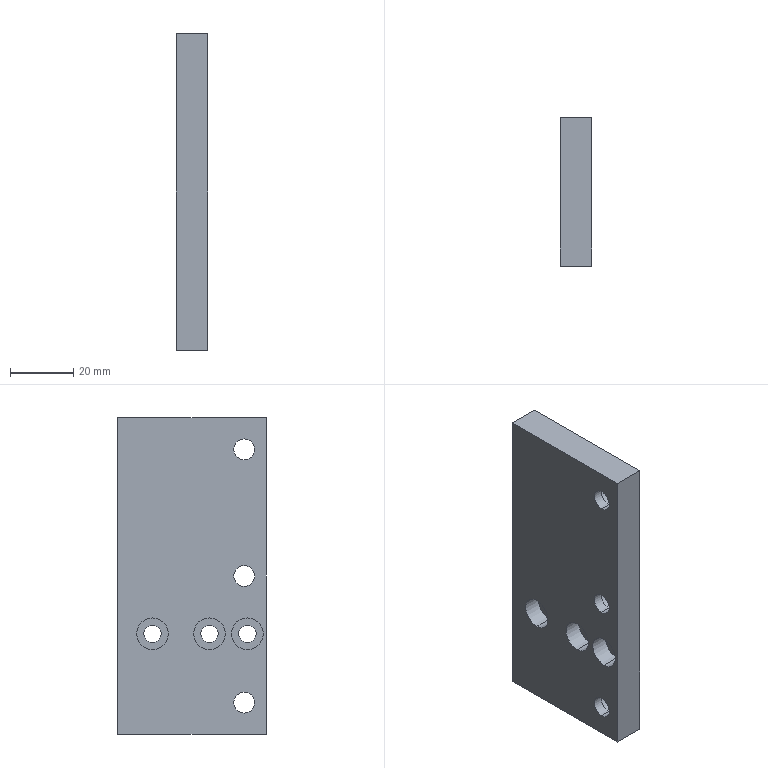Part | SolidWorks | features HoleWzd 3, Extrusion 1 | 1 solid | 44 faces | box 10 x 47 x 100 mm | volume 42728 mm3 | cylinder 28 | plane 12 | cone 4 | commonest cylinder face diameters 5.5 x6 6.6 x6 10 x6 11 x6 4.2 x4
STEP:
#1=CARTESIAN_POINT('',(5.,11.1,27.9));
#2=VERTEX_POINT('',#1);
#3=CARTESIAN_POINT('',(5.,11.1,32.1));
#4=VERTEX_POINT('',#3);
#5=CARTESIAN_POINT('',(5.,11.1,30.));
#6=DIRECTION('',(0.,1.,0.));
#7=DIRECTION('',(0.,0.,1.));
#8=AXIS2_PLACEMENT_3D('',#5,#6,#7);
#9=CIRCLE('',#8,2.1);
#10=EDGE_CURVE('',#2,#4,#9,.T.);
#11=ORIENTED_EDGE('',*,*,#10,.F.);
#12=CARTESIAN_POINT('',(5.,23.5,27.9));
#13=VERTEX_POINT('',#12);
#14=CARTESIAN_POINT('',(5.,23.5,27.9));
#15=DIRECTION('',(0.,1.,0.));
#16=VECTOR('',#15,1000.);
#17=LINE('',#14,#16);
#18=EDGE_CURVE('',#2,#13,#17,.T.);
#19=ORIENTED_EDGE('',*,*,#18,.T.);
#20=CARTESIAN_POINT('',(5.,23.5,32.1));
#21=VERTEX_POINT('',#20);
#22=CARTESIAN_POINT('',(5.,23.5,30.));
#23=DIRECTION('',(0.,1.,0.));
#24=DIRECTION('',(0.,0.,1.));
#25=AXIS2_PLACEMENT_3D('',#22,#23,#24);
#26=CIRCLE('',#25,2.1);
#27=EDGE_CURVE('',#13,#21,#26,.T.);
#28=ORIENTED_EDGE('',*,*,#27,.T.);
#29=CARTESIAN_POINT('',(5.,23.5,32.1));
#30=DIRECTION('',(0.,1.,0.));
#31=VECTOR('',#30,1000.);
#32=LINE('',#29,#31);
#33=EDGE_CURVE('',#4,#21,#32,.T.);
#34=ORIENTED_EDGE('',*,*,#33,.F.);
#35=EDGE_LOOP('',(#11,#19,#28,#34));
#36=FACE_OUTER_BOUND('',#35,.T.);
#37=CARTESIAN_POINT('',(5.,23.5,30.));
#38=DIRECTION('',(0.,1.,0.));
#39=DIRECTION('',(0.,0.,1.));
#40=AXIS2_PLACEMENT_3D('',#37,#38,#39);
#41=CYLINDRICAL_SURFACE('',#40,2.1);
#42=ADVANCED_FACE('',(#36),#41,.F.);
#43=CARTESIAN_POINT('',(5.,9.838,30.));
#44=VERTEX_POINT('',#43);
#45=CARTESIAN_POINT('',(5.,11.1,32.1));
#46=DIRECTION('',(0.,0.515,0.8572));
#47=VECTOR('',#46,1000.);
#48=LINE('',#45,#47);
#49=EDGE_CURVE('',#44,#4,#48,.T.);
#50=ORIENTED_EDGE('',*,*,#49,.F.);
#51=CARTESIAN_POINT('',(5.,11.1,27.9));
#52=DIRECTION('',(0.,0.515,-0.8572));
#53=VECTOR('',#52,1000.);
#54=LINE('',#51,#53);
#55=EDGE_CURVE('',#44,#2,#54,.T.);
#56=ORIENTED_EDGE('',*,*,#55,.T.);
#57=ORIENTED_EDGE('',*,*,#10,.T.);
#58=EDGE_LOOP('',(#50,#56,#57));
#59=FACE_OUTER_BOUND('',#58,.T.);
#60=CARTESIAN_POINT('',(5.,11.1,30.));
#61=DIRECTION('',(0.,1.,0.));
#62=DIRECTION('',(0.,0.,1.));
#63=AXIS2_PLACEMENT_3D('',#60,#61,#62);
#64=CONICAL_SURFACE('',#63,2.1,1.03);
#65=ADVANCED_FACE('',(#59),#64,.F.);
#66=CARTESIAN_POINT('',(5.,11.1,-32.1));
#67=VERTEX_POINT('',#66);
#68=CARTESIAN_POINT('',(5.,11.1,-27.9));
#69=VERTEX_POINT('',#68);
#70=CARTESIAN_POINT('',(5.,11.1,-30.));
#71=DIRECTION('',(0.,1.,0.));
#72=DIRECTION('',(0.,0.,1.));
#73=AXIS2_PLACEMENT_3D('',#70,#71,#72);
#74=CIRCLE('',#73,2.1);
#75=EDGE_CURVE('',#67,#69,#74,.T.);
#76=ORIENTED_EDGE('',*,*,#75,.F.);
#77=CARTESIAN_POINT('',(5.,23.5,-32.1));
#78=VERTEX_POINT('',#77);
#79=CARTESIAN_POINT('',(5.,23.5,-32.1));
#80=DIRECTION('',(0.,1.,0.));
#81=VECTOR('',#80,1000.);
#82=LINE('',#79,#81);
#83=EDGE_CURVE('',#67,#78,#82,.T.);
#84=ORIENTED_EDGE('',*,*,#83,.T.);
#85=CARTESIAN_POINT('',(5.,23.5,-27.9));
#86=VERTEX_POINT('',#85);
#87=CARTESIAN_POINT('',(5.,23.5,-30.));
#88=DIRECTION('',(0.,1.,0.));
#89=DIRECTION('',(0.,0.,1.));
#90=AXIS2_PLACEMENT_3D('',#87,#88,#89);
#91=CIRCLE('',#90,2.1);
#92=EDGE_CURVE('',#78,#86,#91,.T.);
#93=ORIENTED_EDGE('',*,*,#92,.T.);
#94=CARTESIAN_POINT('',(5.,23.5,-27.9));
#95=DIRECTION('',(0.,1.,0.));
#96=VECTOR('',#95,1000.);
#97=LINE('',#94,#96);
#98=EDGE_CURVE('',#69,#86,#97,.T.);
#99=ORIENTED_EDGE('',*,*,#98,.F.);
#100=EDGE_LOOP('',(#76,#84,#93,#99));
#101=FACE_OUTER_BOUND('',#100,.T.);
#102=CARTESIAN_POINT('',(5.,23.5,-30.));
#103=DIRECTION('',(0.,1.,0.));
#104=DIRECTION('',(0.,0.,1.));
#105=AXIS2_PLACEMENT_3D('',#102,#103,#104);
#106=CYLINDRICAL_SURFACE('',#105,2.1);
#107=ADVANCED_FACE('',(#101),#106,.F.);
#108=CARTESIAN_POINT('',(5.,9.838,-30.));
#109=VERTEX_POINT('',#108);
#110=CARTESIAN_POINT('',(5.,11.1,-27.9));
#111=DIRECTION('',(0.,0.515,0.8572));
#112=VECTOR('',#111,1000.);
#113=LINE('',#110,#112);
#114=EDGE_CURVE('',#109,#69,#113,.T.);
#115=ORIENTED_EDGE('',*,*,#114,.F.);
#116=CARTESIAN_POINT('',(5.,11.1,-32.1));
#117=DIRECTION('',(0.,0.515,-0.8572));
#118=VECTOR('',#117,1000.);
#119=LINE('',#116,#118);
#120=EDGE_CURVE('',#109,#67,#119,.T.);
#121=ORIENTED_EDGE('',*,*,#120,.T.);
#122=ORIENTED_EDGE('',*,*,#75,.T.);
#123=EDGE_LOOP('',(#115,#121,#122));
#124=FACE_OUTER_BOUND('',#123,.T.);
#125=CARTESIAN_POINT('',(5.,11.1,-30.));
#126=DIRECTION('',(0.,1.,0.));
#127=DIRECTION('',(0.,0.,1.));
#128=AXIS2_PLACEMENT_3D('',#125,#126,#127);
#129=CONICAL_SURFACE('',#128,2.1,1.03);
#130=ADVANCED_FACE('',(#124),#129,.F.);
#131=CARTESIAN_POINT('',(5.7,12.5,-23.25));
#132=VERTEX_POINT('',#131);
#133=CARTESIAN_POINT('',(5.7,12.5,-13.25));
#134=VERTEX_POINT('',#133);
#135=CARTESIAN_POINT('',(5.7,12.5,-18.25));
#136=DIRECTION('',(-1.,0.,0.));
#137=DIRECTION('',(0.,0.,1.));
#138=AXIS2_PLACEMENT_3D('',#135,#136,#137);
#139=CIRCLE('',#138,5.);
#140=EDGE_CURVE('',#132,#134,#139,.T.);
#141=ORIENTED_EDGE('',*,*,#140,.F.);
#142=CARTESIAN_POINT('',(0.,12.5,-23.25));
#143=VERTEX_POINT('',#142);
#144=CARTESIAN_POINT('',(0.,12.5,-23.25));
#145=DIRECTION('',(-1.,0.,0.));
#146=VECTOR('',#145,1000.);
#147=LINE('',#144,#146);
#148=EDGE_CURVE('',#132,#143,#147,.T.);
#149=ORIENTED_EDGE('',*,*,#148,.T.);
#150=CARTESIAN_POINT('',(0.,12.5,-13.25));
#151=VERTEX_POINT('',#150);
#152=CARTESIAN_POINT('',(0.,12.5,-18.25));
#153=DIRECTION('',(-1.,0.,0.));
#154=DIRECTION('',(0.,0.,1.));
#155=AXIS2_PLACEMENT_3D('',#152,#153,#154);
#156=CIRCLE('',#155,5.);
#157=EDGE_CURVE('',#143,#151,#156,.T.);
#158=ORIENTED_EDGE('',*,*,#157,.T.);
#159=CARTESIAN_POINT('',(0.,12.5,-13.25));
#160=DIRECTION('',(-1.,0.,0.));
#161=VECTOR('',#160,1000.);
#162=LINE('',#159,#161);
#163=EDGE_CURVE('',#134,#151,#162,.T.);
#164=ORIENTED_EDGE('',*,*,#163,.F.);
#165=EDGE_LOOP('',(#141,#149,#158,#164));
#166=FACE_OUTER_BOUND('',#165,.T.);
#167=CARTESIAN_POINT('',(0.,12.5,-18.25));
#168=DIRECTION('',(-1.,0.,0.));
#169=DIRECTION('',(0.,0.,1.));
#170=AXIS2_PLACEMENT_3D('',#167,#168,#169);
#171=CYLINDRICAL_SURFACE('',#170,5.);
#172=ADVANCED_FACE('',(#166),#171,.F.);
#173=CARTESIAN_POINT('',(10.,12.5,-21.));
#174=VERTEX_POINT('',#173);
#175=CARTESIAN_POINT('',(10.,12.5,-15.5));
#176=VERTEX_POINT('',#175);
#177=CARTESIAN_POINT('',(10.,12.5,-18.25));
#178=DIRECTION('',(-1.,0.,0.));
#179=DIRECTION('',(0.,0.,1.));
#180=AXIS2_PLACEMENT_3D('',#177,#178,#179);
#181=CIRCLE('',#180,2.75);
#182=EDGE_CURVE('',#174,#176,#181,.T.);
#183=ORIENTED_EDGE('',*,*,#182,.F.);
#184=CARTESIAN_POINT('',(5.7,12.5,-21.));
#185=VERTEX_POINT('',#184);
#186=CARTESIAN_POINT('',(0.,12.5,-21.));
#187=DIRECTION('',(-1.,0.,0.));
#188=VECTOR('',#187,1000.);
#189=LINE('',#186,#188);
#190=EDGE_CURVE('',#174,#185,#189,.T.);
#191=ORIENTED_EDGE('',*,*,#190,.T.);
#192=CARTESIAN_POINT('',(5.7,12.5,-15.5));
#193=VERTEX_POINT('',#192);
#194=CARTESIAN_POINT('',(5.7,12.5,-18.25));
#195=DIRECTION('',(-1.,0.,0.));
#196=DIRECTION('',(0.,0.,1.));
#197=AXIS2_PLACEMENT_3D('',#194,#195,#196);
#198=CIRCLE('',#197,2.75);
#199=EDGE_CURVE('',#185,#193,#198,.T.);
#200=ORIENTED_EDGE('',*,*,#199,.T.);
#201=CARTESIAN_POINT('',(0.,12.5,-15.5));
#202=DIRECTION('',(-1.,0.,0.));
#203=VECTOR('',#202,1000.);
#204=LINE('',#201,#203);
#205=EDGE_CURVE('',#176,#193,#204,.T.);
#206=ORIENTED_EDGE('',*,*,#205,.F.);
#207=EDGE_LOOP('',(#183,#191,#200,#206));
#208=FACE_OUTER_BOUND('',#207,.T.);
#209=CARTESIAN_POINT('',(0.,12.5,-18.25));
#210=DIRECTION('',(-1.,0.,0.));
#211=DIRECTION('',(0.,0.,1.));
#212=AXIS2_PLACEMENT_3D('',#209,#210,#211);
#213=CYLINDRICAL_SURFACE('',#212,2.75);
#214=ADVANCED_FACE('',(#208),#213,.F.);
#215=CARTESIAN_POINT('',(5.7,-5.5,-23.25));
#216=VERTEX_POINT('',#215);
#217=CARTESIAN_POINT('',(5.7,-5.5,-13.25));
#218=VERTEX_POINT('',#217);
#219=CARTESIAN_POINT('',(5.7,-5.5,-18.25));
#220=DIRECTION('',(-1.,0.,0.));
#221=DIRECTION('',(0.,0.,1.));
#222=AXIS2_PLACEMENT_3D('',#219,#220,#221);
#223=CIRCLE('',#222,5.);
#224=EDGE_CURVE('',#216,#218,#223,.T.);
#225=ORIENTED_EDGE('',*,*,#224,.F.);
#226=CARTESIAN_POINT('',(0.,-5.5,-23.25));
#227=VERTEX_POINT('',#226);
#228=CARTESIAN_POINT('',(0.,-5.5,-23.25));
#229=DIRECTION('',(-1.,0.,0.));
#230=VECTOR('',#229,1000.);
#231=LINE('',#228,#230);
#232=EDGE_CURVE('',#216,#227,#231,.T.);
#233=ORIENTED_EDGE('',*,*,#232,.T.);
#234=CARTESIAN_POINT('',(0.,-5.5,-13.25));
#235=VERTEX_POINT('',#234);
#236=CARTESIAN_POINT('',(0.,-5.5,-18.25));
#237=DIRECTION('',(-1.,0.,0.));
#238=DIRECTION('',(0.,0.,1.));
#239=AXIS2_PLACEMENT_3D('',#236,#237,#238);
#240=CIRCLE('',#239,5.);
#241=EDGE_CURVE('',#227,#235,#240,.T.);
#242=ORIENTED_EDGE('',*,*,#241,.T.);
#243=CARTESIAN_POINT('',(0.,-5.5,-13.25));
#244=DIRECTION('',(-1.,0.,0.));
#245=VECTOR('',#244,1000.);
#246=LINE('',#243,#245);
#247=EDGE_CURVE('',#218,#235,#246,.T.);
#248=ORIENTED_EDGE('',*,*,#247,.F.);
#249=EDGE_LOOP('',(#225,#233,#242,#248));
#250=FACE_OUTER_BOUND('',#249,.T.);
#251=CARTESIAN_POINT('',(0.,-5.5,-18.25));
#252=DIRECTION('',(-1.,0.,0.));
#253=DIRECTION('',(0.,0.,1.));
#254=AXIS2_PLACEMENT_3D('',#251,#252,#253);
#255=CYLINDRICAL_SURFACE('',#254,5.);
#256=ADVANCED_FACE('',(#250),#255,.F.);
#257=CARTESIAN_POINT('',(10.,-5.5,-21.));
#258=VERTEX_POINT('',#257);
#259=CARTESIAN_POINT('',(10.,-5.5,-15.5));
#260=VERTEX_POINT('',#259);
#261=CARTESIAN_POINT('',(10.,-5.5,-18.25));
#262=DIRECTION('',(-1.,0.,0.));
#263=DIRECTION('',(0.,0.,1.));
#264=AXIS2_PLACEMENT_3D('',#261,#262,#263);
#265=CIRCLE('',#264,2.75);
#266=EDGE_CURVE('',#258,#260,#265,.T.);
#267=ORIENTED_EDGE('',*,*,#266,.F.);
#268=CARTESIAN_POINT('',(5.7,-5.5,-21.));
#269=VERTEX_POINT('',#268);
#270=CARTESIAN_POINT('',(0.,-5.5,-21.));
#271=DIRECTION('',(-1.,0.,0.));
#272=VECTOR('',#271,1000.);
#273=LINE('',#270,#272);
#274=EDGE_CURVE('',#258,#269,#273,.T.);
#275=ORIENTED_EDGE('',*,*,#274,.T.);
#276=CARTESIAN_POINT('',(5.7,-5.5,-15.5));
#277=VERTEX_POINT('',#276);
#278=CARTESIAN_POINT('',(5.7,-5.5,-18.25));
#279=DIRECTION('',(-1.,0.,0.));
#280=DIRECTION('',(0.,0.,1.));
#281=AXIS2_PLACEMENT_3D('',#278,#279,#280);
#282=CIRCLE('',#281,2.75);
#283=EDGE_CURVE('',#269,#277,#282,.T.);
#284=ORIENTED_EDGE('',*,*,#283,.T.);
#285=CARTESIAN_POINT('',(0.,-5.5,-15.5));
#286=DIRECTION('',(-1.,0.,0.));
#287=VECTOR('',#286,1000.);
#288=LINE('',#285,#287);
#289=EDGE_CURVE('',#260,#277,#288,.T.);
#290=ORIENTED_EDGE('',*,*,#289,.F.);
#291=EDGE_LOOP('',(#267,#275,#284,#290));
#292=FACE_OUTER_BOUND('',#291,.T.);
#293=CARTESIAN_POINT('',(0.,-5.5,-18.25));
#294=DIRECTION('',(-1.,0.,0.));
#295=DIRECTION('',(0.,0.,1.));
#296=AXIS2_PLACEMENT_3D('',#293,#294,#295);
#297=CYLINDRICAL_SURFACE('',#296,2.75);
#298=ADVANCED_FACE('',(#292),#297,.F.);
#299=CARTESIAN_POINT('',(5.7,-17.5,-23.25));
#300=VERTEX_POINT('',#299);
#301=CARTESIAN_POINT('',(5.7,-17.5,-13.25));
#302=VERTEX_POINT('',#301);
#303=CARTESIAN_POINT('',(5.7,-17.5,-18.25));
#304=DIRECTION('',(-1.,0.,0.));
#305=DIRECTION('',(0.,0.,1.));
#306=AXIS2_PLACEMENT_3D('',#303,#304,#305);
#307=CIRCLE('',#306,5.);
#308=EDGE_CURVE('',#300,#302,#307,.T.);
#309=ORIENTED_EDGE('',*,*,#308,.F.);
#310=CARTESIAN_POINT('',(0.,-17.5,-23.25));
#311=VERTEX_POINT('',#310);
#312=CARTESIAN_POINT('',(0.,-17.5,-23.25));
#313=DIRECTION('',(-1.,0.,0.));
#314=VECTOR('',#313,1000.);
#315=LINE('',#312,#314);
#316=EDGE_CURVE('',#300,#311,#315,.T.);
#317=ORIENTED_EDGE('',*,*,#316,.T.);
#318=CARTESIAN_POINT('',(0.,-17.5,-13.25));
#319=VERTEX_POINT('',#318);
#320=CARTESIAN_POINT('',(0.,-17.5,-18.25));
#321=DIRECTION('',(-1.,0.,0.));
#322=DIRECTION('',(0.,0.,1.));
#323=AXIS2_PLACEMENT_3D('',#320,#321,#322);
#324=CIRCLE('',#323,5.);
#325=EDGE_CURVE('',#311,#319,#324,.T.);
#326=ORIENTED_EDGE('',*,*,#325,.T.);
#327=CARTESIAN_POINT('',(0.,-17.5,-13.25));
#328=DIRECTION('',(-1.,0.,0.));
#329=VECTOR('',#328,1000.);
#330=LINE('',#327,#329);
#331=EDGE_CURVE('',#302,#319,#330,.T.);
#332=ORIENTED_EDGE('',*,*,#331,.F.);
#333=EDGE_LOOP('',(#309,#317,#326,#332));
#334=FACE_OUTER_BOUND('',#333,.T.);
#335=CARTESIAN_POINT('',(0.,-17.5,-18.25));
#336=DIRECTION('',(-1.,0.,0.));
#337=DIRECTION('',(0.,0.,1.));
#338=AXIS2_PLACEMENT_3D('',#335,#336,#337);
#339=CYLINDRICAL_SURFACE('',#338,5.);
#340=ADVANCED_FACE('',(#334),#339,.F.);
#341=CARTESIAN_POINT('',(10.,-17.5,-21.));
#342=VERTEX_POINT('',#341);
#343=CARTESIAN_POINT('',(10.,-17.5,-15.5));
#344=VERTEX_POINT('',#343);
#345=CARTESIAN_POINT('',(10.,-17.5,-18.25));
#346=DIRECTION('',(-1.,0.,0.));
#347=DIRECTION('',(0.,0.,1.));
#348=AXIS2_PLACEMENT_3D('',#345,#346,#347);
#349=CIRCLE('',#348,2.75);
#350=EDGE_CURVE('',#342,#344,#349,.T.);
#351=ORIENTED_EDGE('',*,*,#350,.F.);
#352=CARTESIAN_POINT('',(5.7,-17.5,-21.));
#353=VERTEX_POINT('',#352);
#354=CARTESIAN_POINT('',(0.,-17.5,-21.));
#355=DIRECTION('',(-1.,0.,0.));
#356=VECTOR('',#355,1000.);
#357=LINE('',#354,#356);
#358=EDGE_CURVE('',#342,#353,#357,.T.);
#359=ORIENTED_EDGE('',*,*,#358,.T.);
#360=CARTESIAN_POINT('',(5.7,-17.5,-15.5));
#361=VERTEX_POINT('',#360);
#362=CARTESIAN_POINT('',(5.7,-17.5,-18.25));
#363=DIRECTION('',(-1.,0.,0.));
#364=DIRECTION('',(0.,0.,1.));
#365=AXIS2_PLACEMENT_3D('',#362,#363,#364);
#366=CIRCLE('',#365,2.75);
#367=EDGE_CURVE('',#353,#361,#366,.T.);
#368=ORIENTED_EDGE('',*,*,#367,.T.);
#369=CARTESIAN_POINT('',(0.,-17.5,-15.5));
#370=DIRECTION('',(-1.,0.,0.));
#371=VECTOR('',#370,1000.);
#372=LINE('',#369,#371);
#373=EDGE_CURVE('',#344,#361,#372,.T.);
#374=ORIENTED_EDGE('',*,*,#373,.F.);
#375=EDGE_LOOP('',(#351,#359,#368,#374));
#376=FACE_OUTER_BOUND('',#375,.T.);
#377=CARTESIAN_POINT('',(0.,-17.5,-18.25));
#378=DIRECTION('',(-1.,0.,0.));
#379=DIRECTION('',(0.,0.,1.));
#380=AXIS2_PLACEMENT_3D('',#377,#378,#379);
#381=CYLINDRICAL_SURFACE('',#380,2.75);
#382=ADVANCED_FACE('',(#376),#381,.F.);
#383=CARTESIAN_POINT('',(3.2,-16.5,45.5));
#384=VERTEX_POINT('',#383);
#385=CARTESIAN_POINT('',(3.2,-16.5,34.5));
#386=VERTEX_POINT('',#385);
#387=CARTESIAN_POINT('',(3.2,-16.5,40.));
#388=DIRECTION('',(1.,0.,0.));
#389=DIRECTION('',(0.,0.,-1.));
#390=AXIS2_PLACEMENT_3D('',#387,#388,#389);
#391=CIRCLE('',#390,5.5);
#392=EDGE_CURVE('',#384,#386,#391,.T.);
#393=ORIENTED_EDGE('',*,*,#392,.F.);
#394=CARTESIAN_POINT('',(10.,-16.5,45.5));
#395=VERTEX_POINT('',#394);
#396=CARTESIAN_POINT('',(10.,-16.5,45.5));
#397=DIRECTION('',(1.,0.,0.));
#398=VECTOR('',#397,1000.);
#399=LINE('',#396,#398);
#400=EDGE_CURVE('',#384,#395,#399,.T.);
#401=ORIENTED_EDGE('',*,*,#400,.T.);
#402=CARTESIAN_POINT('',(10.,-16.5,34.5));
#403=VERTEX_POINT('',#402);
#404=CARTESIAN_POINT('',(10.,-16.5,40.));
#405=DIRECTION('',(1.,0.,0.));
#406=DIRECTION('',(0.,0.,-1.));
#407=AXIS2_PLACEMENT_3D('',#404,#405,#406);
#408=CIRCLE('',#407,5.5);
#409=EDGE_CURVE('',#395,#403,#408,.T.);
#410=ORIENTED_EDGE('',*,*,#409,.T.);
#411=CARTESIAN_POINT('',(10.,-16.5,34.5));
#412=DIRECTION('',(1.,0.,0.));
#413=VECTOR('',#412,1000.);
#414=LINE('',#411,#413);
#415=EDGE_CURVE('',#386,#403,#414,.T.);
#416=ORIENTED_EDGE('',*,*,#415,.F.);
#417=EDGE_LOOP('',(#393,#401,#410,#416));
#418=FACE_OUTER_BOUND('',#417,.T.);
#419=CARTESIAN_POINT('',(10.,-16.5,40.));
#420=DIRECTION('',(1.,0.,0.));
#421=DIRECTION('',(0.,0.,-1.));
#422=AXIS2_PLACEMENT_3D('',#419,#420,#421);
#423=CYLINDRICAL_SURFACE('',#422,5.5);
#424=ADVANCED_FACE('',(#418),#423,.F.);
#425=CARTESIAN_POINT('',(0.,-16.5,43.3));
#426=VERTEX_POINT('',#425);
#427=CARTESIAN_POINT('',(0.,-16.5,36.7));
#428=VERTEX_POINT('',#427);
#429=CARTESIAN_POINT('',(0.,-16.5,40.));
#430=DIRECTION('',(1.,0.,0.));
#431=DIRECTION('',(0.,0.,-1.));
#432=AXIS2_PLACEMENT_3D('',#429,#430,#431);
#433=CIRCLE('',#432,3.3);
#434=EDGE_CURVE('',#426,#428,#433,.T.);
#435=ORIENTED_EDGE('',*,*,#434,.F.);
#436=CARTESIAN_POINT('',(3.2,-16.5,43.3));
#437=VERTEX_POINT('',#436);
#438=CARTESIAN_POINT('',(10.,-16.5,43.3));
#439=DIRECTION('',(1.,0.,0.));
#440=VECTOR('',#439,1000.);
#441=LINE('',#438,#440);
#442=EDGE_CURVE('',#426,#437,#441,.T.);
#443=ORIENTED_EDGE('',*,*,#442,.T.);
#444=CARTESIAN_POINT('',(3.2,-16.5,36.7));
#445=VERTEX_POINT('',#444);
#446=CARTESIAN_POINT('',(3.2,-16.5,40.));
#447=DIRECTION('',(1.,0.,0.));
#448=DIRECTION('',(0.,0.,-1.));
#449=AXIS2_PLACEMENT_3D('',#446,#447,#448);
#450=CIRCLE('',#449,3.3);
#451=EDGE_CURVE('',#437,#445,#450,.T.);
#452=ORIENTED_EDGE('',*,*,#451,.T.);
#453=CARTESIAN_POINT('',(10.,-16.5,36.7));
#454=DIRECTION('',(1.,0.,0.));
#455=VECTOR('',#454,1000.);
#456=LINE('',#453,#455);
#457=EDGE_CURVE('',#428,#445,#456,.T.);
#458=ORIENTED_EDGE('',*,*,#457,.F.);
#459=EDGE_LOOP('',(#435,#443,#452,#458));
#460=FACE_OUTER_BOUND('',#459,.T.);
#461=CARTESIAN_POINT('',(10.,-16.5,40.));
#462=DIRECTION('',(1.,0.,0.));
#463=DIRECTION('',(0.,0.,-1.));
#464=AXIS2_PLACEMENT_3D('',#461,#462,#463);
#465=CYLINDRICAL_SURFACE('',#464,3.3);
#466=ADVANCED_FACE('',(#460),#465,.F.);
#467=CARTESIAN_POINT('',(3.2,-16.5,5.5));
#468=VERTEX_POINT('',#467);
#469=CARTESIAN_POINT('',(3.2,-16.5,-5.5));
#470=VERTEX_POINT('',#469);
#471=CARTESIAN_POINT('',(3.2,-16.5,0.));
#472=DIRECTION('',(1.,0.,0.));
#473=DIRECTION('',(0.,0.,-1.));
#474=AXIS2_PLACEMENT_3D('',#471,#472,#473);
#475=CIRCLE('',#474,5.5);
#476=EDGE_CURVE('',#468,#470,#475,.T.);
#477=ORIENTED_EDGE('',*,*,#476,.F.);
#478=CARTESIAN_POINT('',(10.,-16.5,5.5));
#479=VERTEX_POINT('',#478);
#480=CARTESIAN_POINT('',(10.,-16.5,5.5));
#481=DIRECTION('',(1.,0.,0.));
#482=VECTOR('',#481,1000.);
#483=LINE('',#480,#482);
#484=EDGE_CURVE('',#468,#479,#483,.T.);
#485=ORIENTED_EDGE('',*,*,#484,.T.);
#486=CARTESIAN_POINT('',(10.,-16.5,-5.5));
#487=VERTEX_POINT('',#486);
#488=CARTESIAN_POINT('',(10.,-16.5,0.));
#489=DIRECTION('',(1.,0.,0.));
#490=DIRECTION('',(0.,0.,-1.));
#491=AXIS2_PLACEMENT_3D('',#488,#489,#490);
#492=CIRCLE('',#491,5.5);
#493=EDGE_CURVE('',#479,#487,#492,.T.);
#494=ORIENTED_EDGE('',*,*,#493,.T.);
#495=CARTESIAN_POINT('',(10.,-16.5,-5.5));
#496=DIRECTION('',(1.,0.,0.));
#497=VECTOR('',#496,1000.);
#498=LINE('',#495,#497);
#499=EDGE_CURVE('',#470,#487,#498,.T.);
#500=ORIENTED_EDGE('',*,*,#499,.F.);
#501=EDGE_LOOP('',(#477,#485,#494,#500));
#502=FACE_OUTER_BOUND('',#501,.T.);
#503=CARTESIAN_POINT('',(10.,-16.5,0.));
#504=DIRECTION('',(1.,0.,0.));
#505=DIRECTION('',(0.,0.,-1.));
#506=AXIS2_PLACEMENT_3D('',#503,#504,#505);
#507=CYLINDRICAL_SURFACE('',#506,5.5);
#508=ADVANCED_FACE('',(#502),#507,.F.);
#509=CARTESIAN_POINT('',(0.,-16.5,3.3));
#510=VERTEX_POINT('',#509);
#511=CARTESIAN_POINT('',(0.,-16.5,-3.3));
#512=VERTEX_POINT('',#511);
#513=CARTESIAN_POINT('',(0.,-16.5,0.));
#514=DIRECTION('',(1.,0.,0.));
#515=DIRECTION('',(0.,0.,-1.));
#516=AXIS2_PLACEMENT_3D('',#513,#514,#515);
#517=CIRCLE('',#516,3.3);
#518=EDGE_CURVE('',#510,#512,#517,.T.);
#519=ORIENTED_EDGE('',*,*,#518,.F.);
#520=CARTESIAN_POINT('',(3.2,-16.5,3.3));
#521=VERTEX_POINT('',#520);
#522=CARTESIAN_POINT('',(10.,-16.5,3.3));
#523=DIRECTION('',(1.,0.,0.));
#524=VECTOR('',#523,1000.);
#525=LINE('',#522,#524);
#526=EDGE_CURVE('',#510,#521,#525,.T.);
#527=ORIENTED_EDGE('',*,*,#526,.T.);
#528=CARTESIAN_POINT('',(3.2,-16.5,-3.3));
#529=VERTEX_POINT('',#528);
#530=CARTESIAN_POINT('',(3.2,-16.5,0.));
#531=DIRECTION('',(1.,0.,0.));
#532=DIRECTION('',(0.,0.,-1.));
#533=AXIS2_PLACEMENT_3D('',#530,#531,#532);
#534=CIRCLE('',#533,3.3);
#535=EDGE_CURVE('',#521,#529,#534,.T.);
#536=ORIENTED_EDGE('',*,*,#535,.T.);
#537=CARTESIAN_POINT('',(10.,-16.5,-3.3));
#538=DIRECTION('',(1.,0.,0.));
#539=VECTOR('',#538,1000.);
#540=LINE('',#537,#539);
#541=EDGE_CURVE('',#512,#529,#540,.T.);
#542=ORIENTED_EDGE('',*,*,#541,.F.);
#543=EDGE_LOOP('',(#519,#527,#536,#542));
#544=FACE_OUTER_BOUND('',#543,.T.);
#545=CARTESIAN_POINT('',(10.,-16.5,0.));
#546=DIRECTION('',(1.,0.,0.));
#547=DIRECTION('',(0.,0.,-1.));
#548=AXIS2_PLACEMENT_3D('',#545,#546,#547);
#549=CYLINDRICAL_SURFACE('',#548,3.3);
#550=ADVANCED_FACE('',(#544),#549,.F.);
#551=CARTESIAN_POINT('',(3.2,-16.5,-34.5));
#552=VERTEX_POINT('',#551);
#553=CARTESIAN_POINT('',(3.2,-16.5,-45.5));
#554=VERTEX_POINT('',#553);
#555=CARTESIAN_POINT('',(3.2,-16.5,-40.));
#556=DIRECTION('',(1.,0.,0.));
#557=DIRECTION('',(0.,0.,-1.));
#558=AXIS2_PLACEMENT_3D('',#555,#556,#557);
#559=CIRCLE('',#558,5.5);
#560=EDGE_CURVE('',#552,#554,#559,.T.);
#561=ORIENTED_EDGE('',*,*,#560,.F.);
#562=CARTESIAN_POINT('',(10.,-16.5,-34.5));
#563=VERTEX_POINT('',#562);
#564=CARTESIAN_POINT('',(10.,-16.5,-34.5));
#565=DIRECTION('',(1.,0.,0.));
#566=VECTOR('',#565,1000.);
#567=LINE('',#564,#566);
#568=EDGE_CURVE('',#552,#563,#567,.T.);
#569=ORIENTED_EDGE('',*,*,#568,.T.);
#570=CARTESIAN_POINT('',(10.,-16.5,-45.5));
#571=VERTEX_POINT('',#570);
#572=CARTESIAN_POINT('',(10.,-16.5,-40.));
#573=DIRECTION('',(1.,0.,0.));
#574=DIRECTION('',(0.,0.,-1.));
#575=AXIS2_PLACEMENT_3D('',#572,#573,#574);
#576=CIRCLE('',#575,5.5);
#577=EDGE_CURVE('',#563,#571,#576,.T.);
#578=ORIENTED_EDGE('',*,*,#577,.T.);
#579=CARTESIAN_POINT('',(10.,-16.5,-45.5));
#580=DIRECTION('',(1.,0.,0.));
#581=VECTOR('',#580,1000.);
#582=LINE('',#579,#581);
#583=EDGE_CURVE('',#554,#571,#582,.T.);
#584=ORIENTED_EDGE('',*,*,#583,.F.);
#585=EDGE_LOOP('',(#561,#569,#578,#584));
#586=FACE_OUTER_BOUND('',#585,.T.);
#587=CARTESIAN_POINT('',(10.,-16.5,-40.));
#588=DIRECTION('',(1.,0.,0.));
#589=DIRECTION('',(0.,0.,-1.));
#590=AXIS2_PLACEMENT_3D('',#587,#588,#589);
#591=CYLINDRICAL_SURFACE('',#590,5.5);
#592=ADVANCED_FACE('',(#586),#591,.F.);
#593=CARTESIAN_POINT('',(0.,-16.5,-36.7));
#594=VERTEX_POINT('',#593);
#595=CARTESIAN_POINT('',(0.,-16.5,-43.3));
#596=VERTEX_POINT('',#595);
#597=CARTESIAN_POINT('',(0.,-16.5,-40.));
#598=DIRECTION('',(1.,0.,0.));
#599=DIRECTION('',(0.,0.,-1.));
#600=AXIS2_PLACEMENT_3D('',#597,#598,#599);
#601=CIRCLE('',#600,3.3);
#602=EDGE_CURVE('',#594,#596,#601,.T.);
#603=ORIENTED_EDGE('',*,*,#602,.F.);
#604=CARTESIAN_POINT('',(3.2,-16.5,-36.7));
#605=VERTEX_POINT('',#604);
#606=CARTESIAN_POINT('',(10.,-16.5,-36.7));
#607=DIRECTION('',(1.,0.,0.));
#608=VECTOR('',#607,1000.);
#609=LINE('',#606,#608);
#610=EDGE_CURVE('',#594,#605,#609,.T.);
#611=ORIENTED_EDGE('',*,*,#610,.T.);
#612=CARTESIAN_POINT('',(3.2,-16.5,-43.3));
#613=VERTEX_POINT('',#612);
#614=CARTESIAN_POINT('',(3.2,-16.5,-40.));
#615=DIRECTION('',(1.,0.,0.));
#616=DIRECTION('',(0.,0.,-1.));
#617=AXIS2_PLACEMENT_3D('',#614,#615,#616);
#618=CIRCLE('',#617,3.3);
#619=EDGE_CURVE('',#605,#613,#618,.T.);
#620=ORIENTED_EDGE('',*,*,#619,.T.);
#621=CARTESIAN_POINT('',(10.,-16.5,-43.3));
#622=DIRECTION('',(1.,0.,0.));
#623=VECTOR('',#622,1000.);
#624=LINE('',#621,#623);
#625=EDGE_CURVE('',#596,#613,#624,.T.);
#626=ORIENTED_EDGE('',*,*,#625,.F.);
#627=EDGE_LOOP('',(#603,#611,#620,#626));
#628=FACE_OUTER_BOUND('',#627,.T.);
#629=CARTESIAN_POINT('',(10.,-16.5,-40.));
#630=DIRECTION('',(1.,0.,0.));
#631=DIRECTION('',(0.,0.,-1.));
#632=AXIS2_PLACEMENT_3D('',#629,#630,#631);
#633=CYLINDRICAL_SURFACE('',#632,3.3);
#634=ADVANCED_FACE('',(#628),#633,.F.);
#635=CARTESIAN_POINT('',(0.,-23.5,-50.));
#636=VERTEX_POINT('',#635);
#637=CARTESIAN_POINT('',(0.,23.5,-50.));
#638=VERTEX_POINT('',#637);
#639=CARTESIAN_POINT('',(0.,23.5,-50.));
#640=DIRECTION('',(0.,1.,0.));
#641=VECTOR('',#640,1000.);
#642=LINE('',#639,#641);
#643=EDGE_CURVE('',#636,#638,#642,.T.);
#644=ORIENTED_EDGE('',*,*,#643,.T.);
#645=CARTESIAN_POINT('',(10.,23.5,-50.));
#646=VERTEX_POINT('',#645);
#647=CARTESIAN_POINT('',(10.,23.5,-50.));
#648=DIRECTION('',(-1.,0.,0.));
#649=VECTOR('',#648,1000.);
#650=LINE('',#647,#649);
#651=EDGE_CURVE('',#646,#638,#650,.T.);
#652=ORIENTED_EDGE('',*,*,#651,.F.);
#653=CARTESIAN_POINT('',(10.,-23.5,-50.));
#654=VERTEX_POINT('',#653);
#655=CARTESIAN_POINT('',(10.,23.5,-50.));
#656=DIRECTION('',(0.,1.,0.));
#657=VECTOR('',#656,1000.);
#658=LINE('',#655,#657);
#659=EDGE_CURVE('',#654,#646,#658,.T.);
#660=ORIENTED_EDGE('',*,*,#659,.F.);
#661=CARTESIAN_POINT('',(10.,-23.5,-50.));
#662=DIRECTION('',(-1.,0.,0.));
#663=VECTOR('',#662,1000.);
#664=LINE('',#661,#663);
#665=EDGE_CURVE('',#654,#636,#664,.T.);
#666=ORIENTED_EDGE('',*,*,#665,.T.);
#667=EDGE_LOOP('',(#644,#652,#660,#666));
#668=FACE_OUTER_BOUND('',#667,.T.);
#669=CARTESIAN_POINT('',(10.,23.5,-50.));
#670=DIRECTION('',(0.,0.,1.));
#671=DIRECTION('',(0.,-1.,0.));
#672=AXIS2_PLACEMENT_3D('',#669,#670,#671);
#673=PLANE('',#672);
#674=ADVANCED_FACE('',(#668),#673,.F.);
#675=CARTESIAN_POINT('',(5.,23.5,30.));
#676=DIRECTION('',(0.,1.,0.));
#677=DIRECTION('',(0.,0.,1.));
#678=AXIS2_PLACEMENT_3D('',#675,#676,#677);
#679=CIRCLE('',#678,2.1);
#680=EDGE_CURVE('',#21,#13,#679,.T.);
#681=ORIENTED_EDGE('',*,*,#680,.F.);
#682=ORIENTED_EDGE('',*,*,#27,.F.);
#683=EDGE_LOOP('',(#681,#682));
#684=FACE_BOUND('',#683,.T.);
#685=CARTESIAN_POINT('',(5.,23.5,-30.));
#686=DIRECTION('',(0.,1.,0.));
#687=DIRECTION('',(0.,0.,1.));
#688=AXIS2_PLACEMENT_3D('',#685,#686,#687);
#689=CIRCLE('',#688,2.1);
#690=EDGE_CURVE('',#86,#78,#689,.T.);
#691=ORIENTED_EDGE('',*,*,#690,.F.);
#692=ORIENTED_EDGE('',*,*,#92,.F.);
#693=EDGE_LOOP('',(#691,#692));
#694=FACE_BOUND('',#693,.T.);
#695=CARTESIAN_POINT('',(0.,23.5,50.));
#696=VERTEX_POINT('',#695);
#697=CARTESIAN_POINT('',(0.,23.5,50.));
#698=DIRECTION('',(0.,0.,1.));
#699=VECTOR('',#698,1000.);
#700=LINE('',#697,#699);
#701=EDGE_CURVE('',#638,#696,#700,.T.);
#702=ORIENTED_EDGE('',*,*,#701,.T.);
#703=CARTESIAN_POINT('',(10.,23.5,50.));
#704=VERTEX_POINT('',#703);
#705=CARTESIAN_POINT('',(10.,23.5,50.));
#706=DIRECTION('',(-1.,0.,0.));
#707=VECTOR('',#706,1000.);
#708=LINE('',#705,#707);
#709=EDGE_CURVE('',#704,#696,#708,.T.);
#710=ORIENTED_EDGE('',*,*,#709,.F.);
#711=CARTESIAN_POINT('',(10.,23.5,50.));
#712=DIRECTION('',(0.,0.,1.));
#713=VECTOR('',#712,1000.);
#714=LINE('',#711,#713);
#715=EDGE_CURVE('',#646,#704,#714,.T.);
#716=ORIENTED_EDGE('',*,*,#715,.F.);
#717=ORIENTED_EDGE('',*,*,#651,.T.);
#718=EDGE_LOOP('',(#702,#710,#716,#717));
#719=FACE_OUTER_BOUND('',#718,.T.);
#720=CARTESIAN_POINT('',(10.,23.5,50.));
#721=DIRECTION('',(0.,-1.,0.));
#722=DIRECTION('',(0.,0.,-1.));
#723=AXIS2_PLACEMENT_3D('',#720,#721,#722);
#724=PLANE('',#723);
#725=ADVANCED_FACE('',(#684,#694,#719),#724,.F.);
#726=CARTESIAN_POINT('',(0.,-23.5,50.));
#727=VERTEX_POINT('',#726);
#728=CARTESIAN_POINT('',(0.,23.5,50.));
#729=DIRECTION('',(0.,-1.,0.));
#730=VECTOR('',#729,1000.);
#731=LINE('',#728,#730);
#732=EDGE_CURVE('',#696,#727,#731,.T.);
#733=ORIENTED_EDGE('',*,*,#732,.T.);
#734=CARTESIAN_POINT('',(10.,-23.5,50.));
#735=VERTEX_POINT('',#734);
#736=CARTESIAN_POINT('',(10.,-23.5,50.));
#737=DIRECTION('',(-1.,0.,0.));
#738=VECTOR('',#737,1000.);
#739=LINE('',#736,#738);
#740=EDGE_CURVE('',#735,#727,#739,.T.);
#741=ORIENTED_EDGE('',*,*,#740,.F.);
#742=CARTESIAN_POINT('',(10.,23.5,50.));
#743=DIRECTION('',(0.,-1.,0.));
#744=VECTOR('',#743,1000.);
#745=LINE('',#742,#744);
#746=EDGE_CURVE('',#704,#735,#745,.T.);
#747=ORIENTED_EDGE('',*,*,#746,.F.);
#748=ORIENTED_EDGE('',*,*,#709,.T.);
#749=EDGE_LOOP('',(#733,#741,#747,#748));
#750=FACE_OUTER_BOUND('',#749,.T.);
#751=CARTESIAN_POINT('',(10.,23.5,50.));
#752=DIRECTION('',(0.,0.,-1.));
#753=DIRECTION('',(0.,1.,0.));
#754=AXIS2_PLACEMENT_3D('',#751,#752,#753);
#755=PLANE('',#754);
#756=ADVANCED_FACE('',(#750),#755,.F.);
#757=CARTESIAN_POINT('',(0.,-23.5,50.));
#758=DIRECTION('',(0.,0.,-1.));
#759=VECTOR('',#758,1000.);
#760=LINE('',#757,#759);
#761=EDGE_CURVE('',#727,#636,#760,.T.);
#762=ORIENTED_EDGE('',*,*,#761,.T.);
#763=ORIENTED_EDGE('',*,*,#665,.F.);
#764=CARTESIAN_POINT('',(10.,-23.5,50.));
#765=DIRECTION('',(0.,0.,-1.));
#766=VECTOR('',#765,1000.);
#767=LINE('',#764,#766);
#768=EDGE_CURVE('',#735,#654,#767,.T.);
#769=ORIENTED_EDGE('',*,*,#768,.F.);
#770=ORIENTED_EDGE('',*,*,#740,.T.);
#771=EDGE_LOOP('',(#762,#763,#769,#770));
#772=FACE_OUTER_BOUND('',#771,.T.);
#773=CARTESIAN_POINT('',(10.,-23.5,50.));
#774=DIRECTION('',(0.,1.,0.));
#775=DIRECTION('',(0.,0.,1.));
#776=AXIS2_PLACEMENT_3D('',#773,#774,#775);
#777=PLANE('',#776);
#778=ADVANCED_FACE('',(#772),#777,.F.);
#779=CARTESIAN_POINT('',(10.,12.5,-18.25));
#780=DIRECTION('',(-1.,0.,0.));
#781=DIRECTION('',(0.,0.,1.));
#782=AXIS2_PLACEMENT_3D('',#779,#780,#781);
#783=CIRCLE('',#782,2.75);
#784=EDGE_CURVE('',#176,#174,#783,.T.);
#785=ORIENTED_EDGE('',*,*,#784,.T.);
#786=ORIENTED_EDGE('',*,*,#182,.T.);
#787=EDGE_LOOP('',(#785,#786));
#788=FACE_BOUND('',#787,.T.);
#789=CARTESIAN_POINT('',(10.,-5.5,-18.25));
#790=DIRECTION('',(-1.,0.,0.));
#791=DIRECTION('',(0.,0.,1.));
#792=AXIS2_PLACEMENT_3D('',#789,#790,#791);
#793=CIRCLE('',#792,2.75);
#794=EDGE_CURVE('',#260,#258,#793,.T.);
#795=ORIENTED_EDGE('',*,*,#794,.T.);
#796=ORIENTED_EDGE('',*,*,#266,.T.);
#797=EDGE_LOOP('',(#795,#796));
#798=FACE_BOUND('',#797,.T.);
#799=CARTESIAN_POINT('',(10.,-17.5,-18.25));
#800=DIRECTION('',(-1.,0.,0.));
#801=DIRECTION('',(0.,0.,1.));
#802=AXIS2_PLACEMENT_3D('',#799,#800,#801);
#803=CIRCLE('',#802,2.75);
#804=EDGE_CURVE('',#344,#342,#803,.T.);
#805=ORIENTED_EDGE('',*,*,#804,.T.);
#806=ORIENTED_EDGE('',*,*,#350,.T.);
#807=EDGE_LOOP('',(#805,#806));
#808=FACE_BOUND('',#807,.T.);
#809=CARTESIAN_POINT('',(10.,-16.5,40.));
#810=DIRECTION('',(1.,0.,0.));
#811=DIRECTION('',(0.,0.,-1.));
#812=AXIS2_PLACEMENT_3D('',#809,#810,#811);
#813=CIRCLE('',#812,5.5);
#814=EDGE_CURVE('',#403,#395,#813,.T.);
#815=ORIENTED_EDGE('',*,*,#814,.F.);
#816=ORIENTED_EDGE('',*,*,#409,.F.);
#817=EDGE_LOOP('',(#815,#816));
#818=FACE_BOUND('',#817,.T.);
#819=CARTESIAN_POINT('',(10.,-16.5,0.));
#820=DIRECTION('',(1.,0.,0.));
#821=DIRECTION('',(0.,0.,-1.));
#822=AXIS2_PLACEMENT_3D('',#819,#820,#821);
#823=CIRCLE('',#822,5.5);
#824=EDGE_CURVE('',#487,#479,#823,.T.);
#825=ORIENTED_EDGE('',*,*,#824,.F.);
#826=ORIENTED_EDGE('',*,*,#493,.F.);
#827=EDGE_LOOP('',(#825,#826));
#828=FACE_BOUND('',#827,.T.);
#829=CARTESIAN_POINT('',(10.,-16.5,-40.));
#830=DIRECTION('',(1.,0.,0.));
#831=DIRECTION('',(0.,0.,-1.));
#832=AXIS2_PLACEMENT_3D('',#829,#830,#831);
#833=CIRCLE('',#832,5.5);
#834=EDGE_CURVE('',#571,#563,#833,.T.);
#835=ORIENTED_EDGE('',*,*,#834,.F.);
#836=ORIENTED_EDGE('',*,*,#577,.F.);
#837=EDGE_LOOP('',(#835,#836));
#838=FACE_BOUND('',#837,.T.);
#839=ORIENTED_EDGE('',*,*,#659,.T.);
#840=ORIENTED_EDGE('',*,*,#715,.T.);
#841=ORIENTED_EDGE('',*,*,#746,.T.);
#842=ORIENTED_EDGE('',*,*,#768,.T.);
#843=EDGE_LOOP('',(#839,#840,#841,#842));
#844=FACE_OUTER_BOUND('',#843,.T.);
#845=CARTESIAN_POINT('',(10.,0.,0.));
#846=DIRECTION('',(1.,0.,0.));
#847=DIRECTION('',(0.,0.,-1.));
#848=AXIS2_PLACEMENT_3D('',#845,#846,#847);
#849=PLANE('',#848);
#850=ADVANCED_FACE('',(#788,#798,#808,#818,#828,#838,#844),#849,.T.);
#851=CARTESIAN_POINT('',(0.,12.5,-18.25));
#852=DIRECTION('',(-1.,0.,0.));
#853=DIRECTION('',(0.,0.,1.));
#854=AXIS2_PLACEMENT_3D('',#851,#852,#853);
#855=CIRCLE('',#854,5.);
#856=EDGE_CURVE('',#151,#143,#855,.T.);
#857=ORIENTED_EDGE('',*,*,#856,.F.);
#858=ORIENTED_EDGE('',*,*,#157,.F.);
#859=EDGE_LOOP('',(#857,#858));
#860=FACE_BOUND('',#859,.T.);
#861=CARTESIAN_POINT('',(0.,-5.5,-18.25));
#862=DIRECTION('',(-1.,0.,0.));
#863=DIRECTION('',(0.,0.,1.));
#864=AXIS2_PLACEMENT_3D('',#861,#862,#863);
#865=CIRCLE('',#864,5.);
#866=EDGE_CURVE('',#235,#227,#865,.T.);
#867=ORIENTED_EDGE('',*,*,#866,.F.);
#868=ORIENTED_EDGE('',*,*,#241,.F.);
#869=EDGE_LOOP('',(#867,#868));
#870=FACE_BOUND('',#869,.T.);
#871=CARTESIAN_POINT('',(0.,-17.5,-18.25));
#872=DIRECTION('',(-1.,0.,0.));
#873=DIRECTION('',(0.,0.,1.));
#874=AXIS2_PLACEMENT_3D('',#871,#872,#873);
#875=CIRCLE('',#874,5.);
#876=EDGE_CURVE('',#319,#311,#875,.T.);
#877=ORIENTED_EDGE('',*,*,#876,.F.);
#878=ORIENTED_EDGE('',*,*,#325,.F.);
#879=EDGE_LOOP('',(#877,#878));
#880=FACE_BOUND('',#879,.T.);
#881=CARTESIAN_POINT('',(0.,-16.5,40.));
#882=DIRECTION('',(1.,0.,0.));
#883=DIRECTION('',(0.,0.,-1.));
#884=AXIS2_PLACEMENT_3D('',#881,#882,#883);
#885=CIRCLE('',#884,3.3);
#886=EDGE_CURVE('',#428,#426,#885,.T.);
#887=ORIENTED_EDGE('',*,*,#886,.T.);
#888=ORIENTED_EDGE('',*,*,#434,.T.);
#889=EDGE_LOOP('',(#887,#888));
#890=FACE_BOUND('',#889,.T.);
#891=CARTESIAN_POINT('',(0.,-16.5,0.));
#892=DIRECTION('',(1.,0.,0.));
#893=DIRECTION('',(0.,0.,-1.));
#894=AXIS2_PLACEMENT_3D('',#891,#892,#893);
#895=CIRCLE('',#894,3.3);
#896=EDGE_CURVE('',#512,#510,#895,.T.);
#897=ORIENTED_EDGE('',*,*,#896,.T.);
#898=ORIENTED_EDGE('',*,*,#518,.T.);
#899=EDGE_LOOP('',(#897,#898));
#900=FACE_BOUND('',#899,.T.);
#901=CARTESIAN_POINT('',(0.,-16.5,-40.));
#902=DIRECTION('',(1.,0.,0.));
#903=DIRECTION('',(0.,0.,-1.));
#904=AXIS2_PLACEMENT_3D('',#901,#902,#903);
#905=CIRCLE('',#904,3.3);
#906=EDGE_CURVE('',#596,#594,#905,.T.);
#907=ORIENTED_EDGE('',*,*,#906,.T.);
#908=ORIENTED_EDGE('',*,*,#602,.T.);
#909=EDGE_LOOP('',(#907,#908));
#910=FACE_BOUND('',#909,.T.);
#911=ORIENTED_EDGE('',*,*,#643,.F.);
#912=ORIENTED_EDGE('',*,*,#761,.F.);
#913=ORIENTED_EDGE('',*,*,#732,.F.);
#914=ORIENTED_EDGE('',*,*,#701,.F.);
#915=EDGE_LOOP('',(#911,#912,#913,#914));
#916=FACE_OUTER_BOUND('',#915,.T.);
#917=CARTESIAN_POINT('',(0.,0.,0.));
#918=DIRECTION('',(1.,0.,0.));
#919=DIRECTION('',(0.,0.,-1.));
#920=AXIS2_PLACEMENT_3D('',#917,#918,#919);
#921=PLANE('',#920);
#922=ADVANCED_FACE('',(#860,#870,#880,#890,#900,#910,#916),#921,.F.);
#923=ORIENTED_EDGE('',*,*,#610,.F.);
#924=ORIENTED_EDGE('',*,*,#906,.F.);
#925=ORIENTED_EDGE('',*,*,#625,.T.);
#926=CARTESIAN_POINT('',(3.2,-16.5,-40.));
#927=DIRECTION('',(1.,0.,0.));
#928=DIRECTION('',(0.,0.,-1.));
#929=AXIS2_PLACEMENT_3D('',#926,#927,#928);
#930=CIRCLE('',#929,3.3);
#931=EDGE_CURVE('',#613,#605,#930,.T.);
#932=ORIENTED_EDGE('',*,*,#931,.T.);
#933=EDGE_LOOP('',(#923,#924,#925,#932));
#934=FACE_OUTER_BOUND('',#933,.T.);
#935=CARTESIAN_POINT('',(10.,-16.5,-40.));
#936=DIRECTION('',(1.,0.,0.));
#937=DIRECTION('',(0.,0.,-1.));
#938=AXIS2_PLACEMENT_3D('',#935,#936,#937);
#939=CYLINDRICAL_SURFACE('',#938,3.3);
#940=ADVANCED_FACE('',(#934),#939,.F.);
#941=ORIENTED_EDGE('',*,*,#931,.F.);
#942=ORIENTED_EDGE('',*,*,#619,.F.);
#943=EDGE_LOOP('',(#941,#942));
#944=FACE_BOUND('',#943,.T.);
#945=CARTESIAN_POINT('',(3.2,-16.5,-40.));
#946=DIRECTION('',(1.,0.,0.));
#947=DIRECTION('',(0.,0.,-1.));
#948=AXIS2_PLACEMENT_3D('',#945,#946,#947);
#949=CIRCLE('',#948,5.5);
#950=EDGE_CURVE('',#554,#552,#949,.T.);
#951=ORIENTED_EDGE('',*,*,#950,.T.);
#952=ORIENTED_EDGE('',*,*,#560,.T.);
#953=EDGE_LOOP('',(#951,#952));
#954=FACE_OUTER_BOUND('',#953,.T.);
#955=CARTESIAN_POINT('',(3.2,-13.2,-40.));
#956=DIRECTION('',(-1.,0.,0.));
#957=DIRECTION('',(0.,0.,1.));
#958=AXIS2_PLACEMENT_3D('',#955,#956,#957);
#959=PLANE('',#958);
#960=ADVANCED_FACE('',(#944,#954),#959,.F.);
#961=ORIENTED_EDGE('',*,*,#568,.F.);
#962=ORIENTED_EDGE('',*,*,#950,.F.);
#963=ORIENTED_EDGE('',*,*,#583,.T.);
#964=ORIENTED_EDGE('',*,*,#834,.T.);
#965=EDGE_LOOP('',(#961,#962,#963,#964));
#966=FACE_OUTER_BOUND('',#965,.T.);
#967=CARTESIAN_POINT('',(10.,-16.5,-40.));
#968=DIRECTION('',(1.,0.,0.));
#969=DIRECTION('',(0.,0.,-1.));
#970=AXIS2_PLACEMENT_3D('',#967,#968,#969);
#971=CYLINDRICAL_SURFACE('',#970,5.5);
#972=ADVANCED_FACE('',(#966),#971,.F.);
#973=ORIENTED_EDGE('',*,*,#526,.F.);
#974=ORIENTED_EDGE('',*,*,#896,.F.);
#975=ORIENTED_EDGE('',*,*,#541,.T.);
#976=CARTESIAN_POINT('',(3.2,-16.5,0.));
#977=DIRECTION('',(1.,0.,0.));
#978=DIRECTION('',(0.,0.,-1.));
#979=AXIS2_PLACEMENT_3D('',#976,#977,#978);
#980=CIRCLE('',#979,3.3);
#981=EDGE_CURVE('',#529,#521,#980,.T.);
#982=ORIENTED_EDGE('',*,*,#981,.T.);
#983=EDGE_LOOP('',(#973,#974,#975,#982));
#984=FACE_OUTER_BOUND('',#983,.T.);
#985=CARTESIAN_POINT('',(10.,-16.5,0.));
#986=DIRECTION('',(1.,0.,0.));
#987=DIRECTION('',(0.,0.,-1.));
#988=AXIS2_PLACEMENT_3D('',#985,#986,#987);
#989=CYLINDRICAL_SURFACE('',#988,3.3);
#990=ADVANCED_FACE('',(#984),#989,.F.);
#991=ORIENTED_EDGE('',*,*,#981,.F.);
#992=ORIENTED_EDGE('',*,*,#535,.F.);
#993=EDGE_LOOP('',(#991,#992));
#994=FACE_BOUND('',#993,.T.);
#995=CARTESIAN_POINT('',(3.2,-16.5,0.));
#996=DIRECTION('',(1.,0.,0.));
#997=DIRECTION('',(0.,0.,-1.));
#998=AXIS2_PLACEMENT_3D('',#995,#996,#997);
#999=CIRCLE('',#998,5.5);
#1000=EDGE_CURVE('',#470,#468,#999,.T.);
#1001=ORIENTED_EDGE('',*,*,#1000,.T.);
#1002=ORIENTED_EDGE('',*,*,#476,.T.);
#1003=EDGE_LOOP('',(#1001,#1002));
#1004=FACE_OUTER_BOUND('',#1003,.T.);
#1005=CARTESIAN_POINT('',(3.2,-13.2,0.));
#1006=DIRECTION('',(-1.,0.,0.));
#1007=DIRECTION('',(0.,0.,1.));
#1008=AXIS2_PLACEMENT_3D('',#1005,#1006,#1007);
#1009=PLANE('',#1008);
#1010=ADVANCED_FACE('',(#994,#1004),#1009,.F.);
#1011=ORIENTED_EDGE('',*,*,#484,.F.);
#1012=ORIENTED_EDGE('',*,*,#1000,.F.);
#1013=ORIENTED_EDGE('',*,*,#499,.T.);
#1014=ORIENTED_EDGE('',*,*,#824,.T.);
#1015=EDGE_LOOP('',(#1011,#1012,#1013,#1014));
#1016=FACE_OUTER_BOUND('',#1015,.T.);
#1017=CARTESIAN_POINT('',(10.,-16.5,0.));
#1018=DIRECTION('',(1.,0.,0.));
#1019=DIRECTION('',(0.,0.,-1.));
#1020=AXIS2_PLACEMENT_3D('',#1017,#1018,#1019);
#1021=CYLINDRICAL_SURFACE('',#1020,5.5);
#1022=ADVANCED_FACE('',(#1016),#1021,.F.);
#1023=ORIENTED_EDGE('',*,*,#442,.F.);
#1024=ORIENTED_EDGE('',*,*,#886,.F.);
#1025=ORIENTED_EDGE('',*,*,#457,.T.);
#1026=CARTESIAN_POINT('',(3.2,-16.5,40.));
#1027=DIRECTION('',(1.,0.,0.));
#1028=DIRECTION('',(0.,0.,-1.));
#1029=AXIS2_PLACEMENT_3D('',#1026,#1027,#1028);
#1030=CIRCLE('',#1029,3.3);
#1031=EDGE_CURVE('',#445,#437,#1030,.T.);
#1032=ORIENTED_EDGE('',*,*,#1031,.T.);
#1033=EDGE_LOOP('',(#1023,#1024,#1025,#1032));
#1034=FACE_OUTER_BOUND('',#1033,.T.);
#1035=CARTESIAN_POINT('',(10.,-16.5,40.));
#1036=DIRECTION('',(1.,0.,0.));
#1037=DIRECTION('',(0.,0.,-1.));
#1038=AXIS2_PLACEMENT_3D('',#1035,#1036,#1037);
#1039=CYLINDRICAL_SURFACE('',#1038,3.3);
#1040=ADVANCED_FACE('',(#1034),#1039,.F.);
#1041=ORIENTED_EDGE('',*,*,#1031,.F.);
#1042=ORIENTED_EDGE('',*,*,#451,.F.);
#1043=EDGE_LOOP('',(#1041,#1042));
#1044=FACE_BOUND('',#1043,.T.);
#1045=CARTESIAN_POINT('',(3.2,-16.5,40.));
#1046=DIRECTION('',(1.,0.,0.));
#1047=DIRECTION('',(0.,0.,-1.));
#1048=AXIS2_PLACEMENT_3D('',#1045,#1046,#1047);
#1049=CIRCLE('',#1048,5.5);
#1050=EDGE_CURVE('',#386,#384,#1049,.T.);
#1051=ORIENTED_EDGE('',*,*,#1050,.T.);
#1052=ORIENTED_EDGE('',*,*,#392,.T.);
#1053=EDGE_LOOP('',(#1051,#1052));
#1054=FACE_OUTER_BOUND('',#1053,.T.);
#1055=CARTESIAN_POINT('',(3.2,-13.2,40.));
#1056=DIRECTION('',(-1.,0.,0.));
#1057=DIRECTION('',(0.,0.,1.));
#1058=AXIS2_PLACEMENT_3D('',#1055,#1056,#1057);
#1059=PLANE('',#1058);
#1060=ADVANCED_FACE('',(#1044,#1054),#1059,.F.);
#1061=ORIENTED_EDGE('',*,*,#400,.F.);
#1062=ORIENTED_EDGE('',*,*,#1050,.F.);
#1063=ORIENTED_EDGE('',*,*,#415,.T.);
#1064=ORIENTED_EDGE('',*,*,#814,.T.);
#1065=EDGE_LOOP('',(#1061,#1062,#1063,#1064));
#1066=FACE_OUTER_BOUND('',#1065,.T.);
#1067=CARTESIAN_POINT('',(10.,-16.5,40.));
#1068=DIRECTION('',(1.,0.,0.));
#1069=DIRECTION('',(0.,0.,-1.));
#1070=AXIS2_PLACEMENT_3D('',#1067,#1068,#1069);
#1071=CYLINDRICAL_SURFACE('',#1070,5.5);
#1072=ADVANCED_FACE('',(#1066),#1071,.F.);
#1073=ORIENTED_EDGE('',*,*,#358,.F.);
#1074=ORIENTED_EDGE('',*,*,#804,.F.);
#1075=ORIENTED_EDGE('',*,*,#373,.T.);
#1076=CARTESIAN_POINT('',(5.7,-17.5,-18.25));
#1077=DIRECTION('',(-1.,0.,0.));
#1078=DIRECTION('',(0.,0.,1.));
#1079=AXIS2_PLACEMENT_3D('',#1076,#1077,#1078);
#1080=CIRCLE('',#1079,2.75);
#1081=EDGE_CURVE('',#361,#353,#1080,.T.);
#1082=ORIENTED_EDGE('',*,*,#1081,.T.);
#1083=EDGE_LOOP('',(#1073,#1074,#1075,#1082));
#1084=FACE_OUTER_BOUND('',#1083,.T.);
#1085=CARTESIAN_POINT('',(0.,-17.5,-18.25));
#1086=DIRECTION('',(-1.,0.,0.));
#1087=DIRECTION('',(0.,0.,1.));
#1088=AXIS2_PLACEMENT_3D('',#1085,#1086,#1087);
#1089=CYLINDRICAL_SURFACE('',#1088,2.75);
#1090=ADVANCED_FACE('',(#1084),#1089,.F.);
#1091=ORIENTED_EDGE('',*,*,#1081,.F.);
#1092=ORIENTED_EDGE('',*,*,#367,.F.);
#1093=EDGE_LOOP('',(#1091,#1092));
#1094=FACE_BOUND('',#1093,.T.);
#1095=CARTESIAN_POINT('',(5.7,-17.5,-18.25));
#1096=DIRECTION('',(-1.,0.,0.));
#1097=DIRECTION('',(0.,0.,1.));
#1098=AXIS2_PLACEMENT_3D('',#1095,#1096,#1097);
#1099=CIRCLE('',#1098,5.);
#1100=EDGE_CURVE('',#302,#300,#1099,.T.);
#1101=ORIENTED_EDGE('',*,*,#1100,.T.);
#1102=ORIENTED_EDGE('',*,*,#308,.T.);
#1103=EDGE_LOOP('',(#1101,#1102));
#1104=FACE_OUTER_BOUND('',#1103,.T.);
#1105=CARTESIAN_POINT('',(5.7,-14.75,-18.25));
#1106=DIRECTION('',(1.,0.,0.));
#1107=DIRECTION('',(0.,0.,-1.));
#1108=AXIS2_PLACEMENT_3D('',#1105,#1106,#1107);
#1109=PLANE('',#1108);
#1110=ADVANCED_FACE('',(#1094,#1104),#1109,.F.);
#1111=ORIENTED_EDGE('',*,*,#316,.F.);
#1112=ORIENTED_EDGE('',*,*,#1100,.F.);
#1113=ORIENTED_EDGE('',*,*,#331,.T.);
#1114=ORIENTED_EDGE('',*,*,#876,.T.);
#1115=EDGE_LOOP('',(#1111,#1112,#1113,#1114));
#1116=FACE_OUTER_BOUND('',#1115,.T.);
#1117=CARTESIAN_POINT('',(0.,-17.5,-18.25));
#1118=DIRECTION('',(-1.,0.,0.));
#1119=DIRECTION('',(0.,0.,1.));
#1120=AXIS2_PLACEMENT_3D('',#1117,#1118,#1119);
#1121=CYLINDRICAL_SURFACE('',#1120,5.);
#1122=ADVANCED_FACE('',(#1116),#1121,.F.);
#1123=ORIENTED_EDGE('',*,*,#274,.F.);
#1124=ORIENTED_EDGE('',*,*,#794,.F.);
#1125=ORIENTED_EDGE('',*,*,#289,.T.);
#1126=CARTESIAN_POINT('',(5.7,-5.5,-18.25));
#1127=DIRECTION('',(-1.,0.,0.));
#1128=DIRECTION('',(0.,0.,1.));
#1129=AXIS2_PLACEMENT_3D('',#1126,#1127,#1128);
#1130=CIRCLE('',#1129,2.75);
#1131=EDGE_CURVE('',#277,#269,#1130,.T.);
#1132=ORIENTED_EDGE('',*,*,#1131,.T.);
#1133=EDGE_LOOP('',(#1123,#1124,#1125,#1132));
#1134=FACE_OUTER_BOUND('',#1133,.T.);
#1135=CARTESIAN_POINT('',(0.,-5.5,-18.25));
#1136=DIRECTION('',(-1.,0.,0.));
#1137=DIRECTION('',(0.,0.,1.));
#1138=AXIS2_PLACEMENT_3D('',#1135,#1136,#1137);
#1139=CYLINDRICAL_SURFACE('',#1138,2.75);
#1140=ADVANCED_FACE('',(#1134),#1139,.F.);
#1141=ORIENTED_EDGE('',*,*,#1131,.F.);
#1142=ORIENTED_EDGE('',*,*,#283,.F.);
#1143=EDGE_LOOP('',(#1141,#1142));
#1144=FACE_BOUND('',#1143,.T.);
#1145=CARTESIAN_POINT('',(5.7,-5.5,-18.25));
#1146=DIRECTION('',(-1.,0.,0.));
#1147=DIRECTION('',(0.,0.,1.));
#1148=AXIS2_PLACEMENT_3D('',#1145,#1146,#1147);
#1149=CIRCLE('',#1148,5.);
#1150=EDGE_CURVE('',#218,#216,#1149,.T.);
#1151=ORIENTED_EDGE('',*,*,#1150,.T.);
#1152=ORIENTED_EDGE('',*,*,#224,.T.);
#1153=EDGE_LOOP('',(#1151,#1152));
#1154=FACE_OUTER_BOUND('',#1153,.T.);
#1155=CARTESIAN_POINT('',(5.7,-2.75,-18.25));
#1156=DIRECTION('',(1.,0.,0.));
#1157=DIRECTION('',(0.,0.,-1.));
#1158=AXIS2_PLACEMENT_3D('',#1155,#1156,#1157);
#1159=PLANE('',#1158);
#1160=ADVANCED_FACE('',(#1144,#1154),#1159,.F.);
#1161=ORIENTED_EDGE('',*,*,#232,.F.);
#1162=ORIENTED_EDGE('',*,*,#1150,.F.);
#1163=ORIENTED_EDGE('',*,*,#247,.T.);
#1164=ORIENTED_EDGE('',*,*,#866,.T.);
#1165=EDGE_LOOP('',(#1161,#1162,#1163,#1164));
#1166=FACE_OUTER_BOUND('',#1165,.T.);
#1167=CARTESIAN_POINT('',(0.,-5.5,-18.25));
#1168=DIRECTION('',(-1.,0.,0.));
#1169=DIRECTION('',(0.,0.,1.));
#1170=AXIS2_PLACEMENT_3D('',#1167,#1168,#1169);
#1171=CYLINDRICAL_SURFACE('',#1170,5.);
#1172=ADVANCED_FACE('',(#1166),#1171,.F.);
#1173=ORIENTED_EDGE('',*,*,#190,.F.);
#1174=ORIENTED_EDGE('',*,*,#784,.F.);
#1175=ORIENTED_EDGE('',*,*,#205,.T.);
#1176=CARTESIAN_POINT('',(5.7,12.5,-18.25));
#1177=DIRECTION('',(-1.,0.,0.));
#1178=DIRECTION('',(0.,0.,1.));
#1179=AXIS2_PLACEMENT_3D('',#1176,#1177,#1178);
#1180=CIRCLE('',#1179,2.75);
#1181=EDGE_CURVE('',#193,#185,#1180,.T.);
#1182=ORIENTED_EDGE('',*,*,#1181,.T.);
#1183=EDGE_LOOP('',(#1173,#1174,#1175,#1182));
#1184=FACE_OUTER_BOUND('',#1183,.T.);
#1185=CARTESIAN_POINT('',(0.,12.5,-18.25));
#1186=DIRECTION('',(-1.,0.,0.));
#1187=DIRECTION('',(0.,0.,1.));
#1188=AXIS2_PLACEMENT_3D('',#1185,#1186,#1187);
#1189=CYLINDRICAL_SURFACE('',#1188,2.75);
#1190=ADVANCED_FACE('',(#1184),#1189,.F.);
#1191=ORIENTED_EDGE('',*,*,#1181,.F.);
#1192=ORIENTED_EDGE('',*,*,#199,.F.);
#1193=EDGE_LOOP('',(#1191,#1192));
#1194=FACE_BOUND('',#1193,.T.);
#1195=CARTESIAN_POINT('',(5.7,12.5,-18.25));
#1196=DIRECTION('',(-1.,0.,0.));
#1197=DIRECTION('',(0.,0.,1.));
#1198=AXIS2_PLACEMENT_3D('',#1195,#1196,#1197);
#1199=CIRCLE('',#1198,5.);
#1200=EDGE_CURVE('',#134,#132,#1199,.T.);
#1201=ORIENTED_EDGE('',*,*,#1200,.T.);
#1202=ORIENTED_EDGE('',*,*,#140,.T.);
#1203=EDGE_LOOP('',(#1201,#1202));
#1204=FACE_OUTER_BOUND('',#1203,.T.);
#1205=CARTESIAN_POINT('',(5.7,15.25,-18.25));
#1206=DIRECTION('',(1.,0.,0.));
#1207=DIRECTION('',(0.,0.,-1.));
#1208=AXIS2_PLACEMENT_3D('',#1205,#1206,#1207);
#1209=PLANE('',#1208);
#1210=ADVANCED_FACE('',(#1194,#1204),#1209,.F.);
#1211=ORIENTED_EDGE('',*,*,#148,.F.);
#1212=ORIENTED_EDGE('',*,*,#1200,.F.);
#1213=ORIENTED_EDGE('',*,*,#163,.T.);
#1214=ORIENTED_EDGE('',*,*,#856,.T.);
#1215=EDGE_LOOP('',(#1211,#1212,#1213,#1214));
#1216=FACE_OUTER_BOUND('',#1215,.T.);
#1217=CARTESIAN_POINT('',(0.,12.5,-18.25));
#1218=DIRECTION('',(-1.,0.,0.));
#1219=DIRECTION('',(0.,0.,1.));
#1220=AXIS2_PLACEMENT_3D('',#1217,#1218,#1219);
#1221=CYLINDRICAL_SURFACE('',#1220,5.);
#1222=ADVANCED_FACE('',(#1216),#1221,.F.);
#1223=ORIENTED_EDGE('',*,*,#120,.F.);
#1224=ORIENTED_EDGE('',*,*,#114,.T.);
#1225=CARTESIAN_POINT('',(5.,11.1,-30.));
#1226=DIRECTION('',(0.,1.,0.));
#1227=DIRECTION('',(0.,0.,1.));
#1228=AXIS2_PLACEMENT_3D('',#1225,#1226,#1227);
#1229=CIRCLE('',#1228,2.1);
#1230=EDGE_CURVE('',#69,#67,#1229,.T.);
#1231=ORIENTED_EDGE('',*,*,#1230,.T.);
#1232=EDGE_LOOP('',(#1223,#1224,#1231));
#1233=FACE_OUTER_BOUND('',#1232,.T.);
#1234=CARTESIAN_POINT('',(5.,11.1,-30.));
#1235=DIRECTION('',(0.,1.,0.));
#1236=DIRECTION('',(0.,0.,1.));
#1237=AXIS2_PLACEMENT_3D('',#1234,#1235,#1236);
#1238=CONICAL_SURFACE('',#1237,2.1,1.03);
#1239=ADVANCED_FACE('',(#1233),#1238,.F.);
#1240=ORIENTED_EDGE('',*,*,#83,.F.);
#1241=ORIENTED_EDGE('',*,*,#1230,.F.);
#1242=ORIENTED_EDGE('',*,*,#98,.T.);
#1243=ORIENTED_EDGE('',*,*,#690,.T.);
#1244=EDGE_LOOP('',(#1240,#1241,#1242,#1243));
#1245=FACE_OUTER_BOUND('',#1244,.T.);
#1246=CARTESIAN_POINT('',(5.,23.5,-30.));
#1247=DIRECTION('',(0.,1.,0.));
#1248=DIRECTION('',(0.,0.,1.));
#1249=AXIS2_PLACEMENT_3D('',#1246,#1247,#1248);
#1250=CYLINDRICAL_SURFACE('',#1249,2.1);
#1251=ADVANCED_FACE('',(#1245),#1250,.F.);
#1252=ORIENTED_EDGE('',*,*,#55,.F.);
#1253=ORIENTED_EDGE('',*,*,#49,.T.);
#1254=CARTESIAN_POINT('',(5.,11.1,30.));
#1255=DIRECTION('',(0.,1.,0.));
#1256=DIRECTION('',(0.,0.,1.));
#1257=AXIS2_PLACEMENT_3D('',#1254,#1255,#1256);
#1258=CIRCLE('',#1257,2.1);
#1259=EDGE_CURVE('',#4,#2,#1258,.T.);
#1260=ORIENTED_EDGE('',*,*,#1259,.T.);
#1261=EDGE_LOOP('',(#1252,#1253,#1260));
#1262=FACE_OUTER_BOUND('',#1261,.T.);
#1263=CARTESIAN_POINT('',(5.,11.1,30.));
#1264=DIRECTION('',(0.,1.,0.));
#1265=DIRECTION('',(0.,0.,1.));
#1266=AXIS2_PLACEMENT_3D('',#1263,#1264,#1265);
#1267=CONICAL_SURFACE('',#1266,2.1,1.03);
#1268=ADVANCED_FACE('',(#1262),#1267,.F.);
#1269=ORIENTED_EDGE('',*,*,#18,.F.);
#1270=ORIENTED_EDGE('',*,*,#1259,.F.);
#1271=ORIENTED_EDGE('',*,*,#33,.T.);
#1272=ORIENTED_EDGE('',*,*,#680,.T.);
#1273=EDGE_LOOP('',(#1269,#1270,#1271,#1272));
#1274=FACE_OUTER_BOUND('',#1273,.T.);
#1275=CARTESIAN_POINT('',(5.,23.5,30.));
#1276=DIRECTION('',(0.,1.,0.));
#1277=DIRECTION('',(0.,0.,1.));
#1278=AXIS2_PLACEMENT_3D('',#1275,#1276,#1277);
#1279=CYLINDRICAL_SURFACE('',#1278,2.1);
#1280=ADVANCED_FACE('',(#1274),#1279,.F.);
#1281=CLOSED_SHELL('',(#42,#65,#107,#130,#172,#214,#256,#298,#340,#382,#424,#466,#508,#550,#592,#634,#674,#725,#756,#778,#850,#922,#940,#960,#972,#990,#1010,#1022,#1040,#1060,#1072,#1090,#1110,#1122,#1140,#1160,#1172,#1190,#1210,#1222,#1239,#1251,#1268,#1280));
#1282=MANIFOLD_SOLID_BREP('',#1281);
#1283=CARTESIAN_POINT('',(0.,0.,0.));
#1284=DIRECTION('',(0.,0.,1.));
#1285=DIRECTION('',(1.,0.,0.));
#1286=AXIS2_PLACEMENT_3D('',#1283,#1284,#1285);
#1287=(LENGTH_UNIT()NAMED_UNIT(*)SI_UNIT(.MILLI.,.METRE.));
#1288=UNCERTAINTY_MEASURE_WITH_UNIT(LENGTH_MEASURE(0.00001),#1287,'','');
#1289=(NAMED_UNIT(*)PLANE_ANGLE_UNIT()SI_UNIT($,.RADIAN.));
#1290=(NAMED_UNIT(*)SI_UNIT($,.STERADIAN.)SOLID_ANGLE_UNIT());
#1291=(GEOMETRIC_REPRESENTATION_CONTEXT(3)GLOBAL_UNCERTAINTY_ASSIGNED_CONTEXT((#1288))GLOBAL_UNIT_ASSIGNED_CONTEXT((#1287,#1289,#1290))REPRESENTATION_CONTEXT('',''));
#1292=ADVANCED_BREP_SHAPE_REPRESENTATION('',(#1282,#1286),#1291);